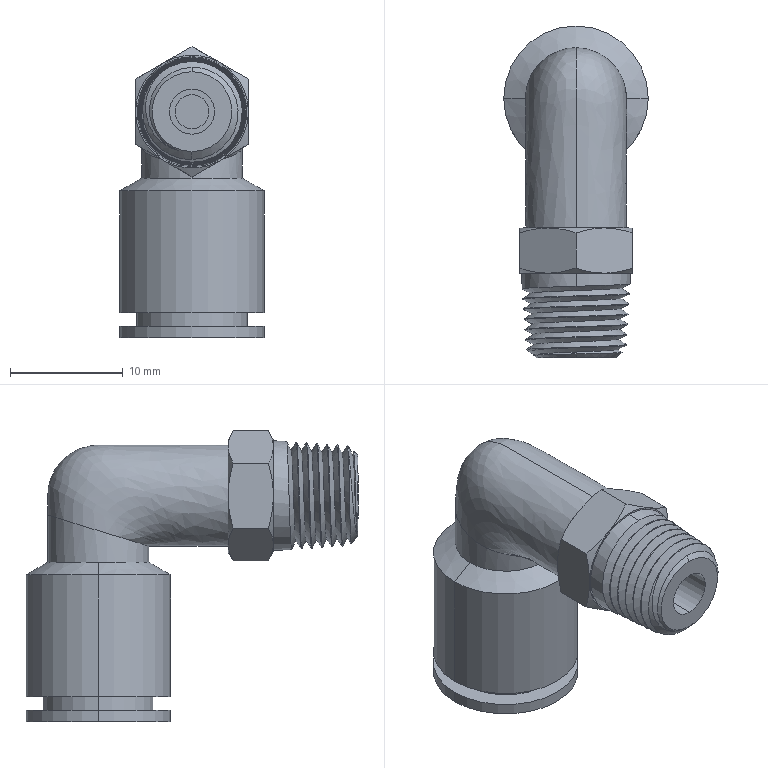Part | 1 solid | 74 faces | box 12.8 x 29.4 x 25.774 mm | volume 2990 mm3 | cone 30 | plane 20 | cylinder 18 | spline 6 | commonest cylinder face diameters 12.8 x4 3 x2 4 x2 6 x2 9.8 x2 10 x2